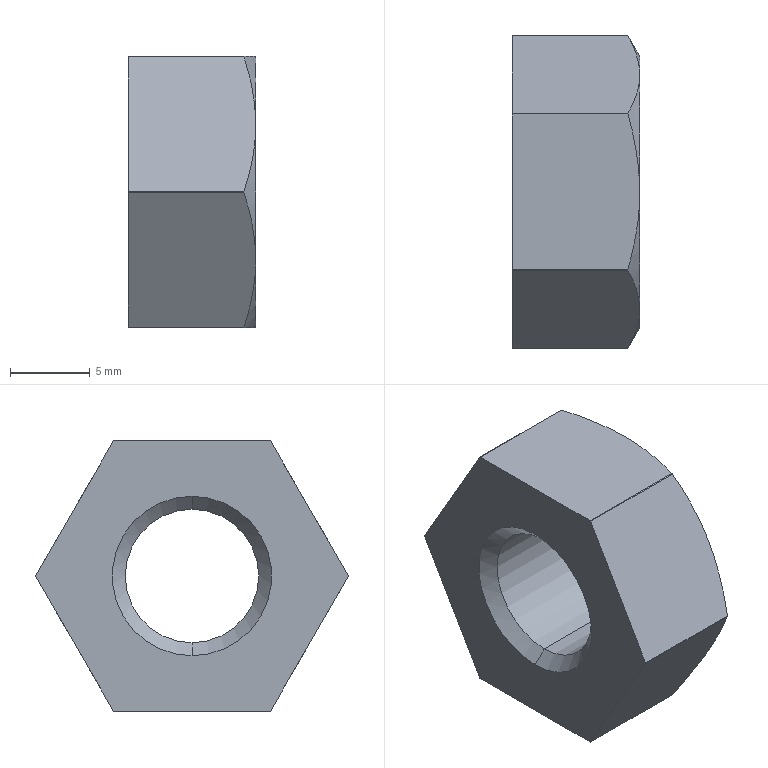Part | STEP file | 2_5 | 1 solid | 26 faces | box 8 x 19.6 x 17 mm | volume 1538 mm3 | cone 10 | cylinder 8 | plane 8 | commonest cylinder face diameters 19.6 x6 8.376 x2